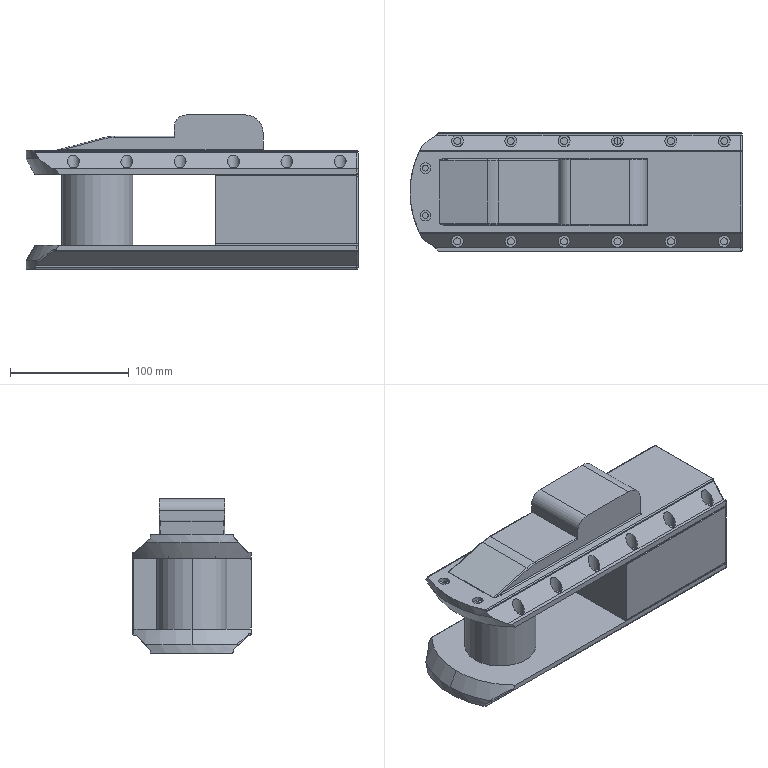Part | SolidWorks | features ICE 13, Fillet 4, Chamfer 3, LPattern 2, 3DProfileFeature 1, Extrusion 1, HoleWzd 1 | 1 solid | 200 faces | box 280 x 100 x 130 mm | volume 1901743 mm3 | cylinder 116 | plane 63 | torus 6 | spline 6 | sphere 6 | cone 3 | commonest cylinder face diameters 2 x45 10 x30 6 x24 4.8 x4 9 x4 60 x4